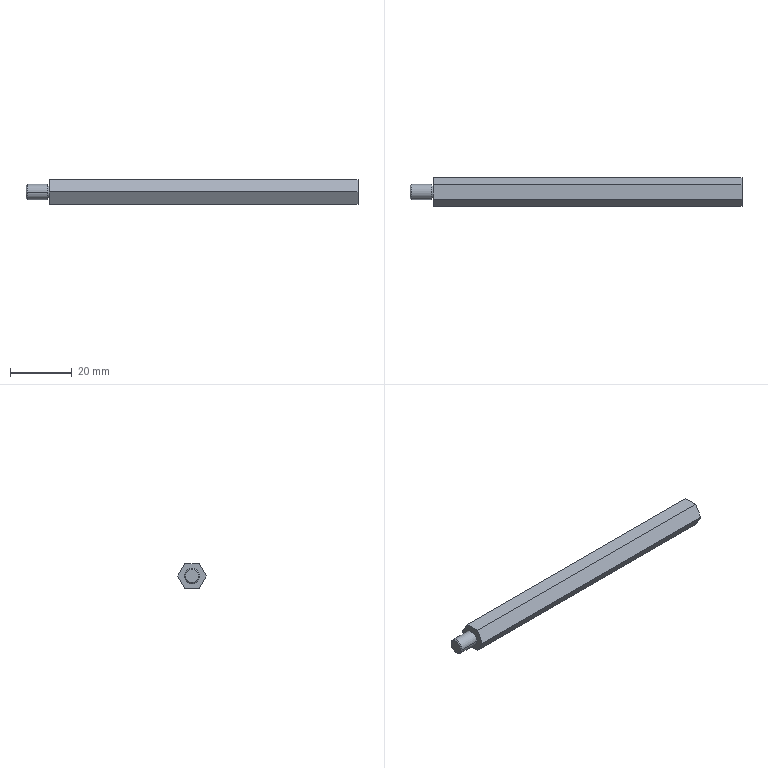Part | NX | 1 solid | 22 faces | box 107.5 x 9.238 x 8 mm | volume 5473 mm3 | plane 10 | cylinder 6 | cone 6 | commonest cylinder face diameters 4.1 x2 4.2 x2 5 x2
STEP:
#1=CARTESIAN_POINT('',(0.,4.619,0.));
#2=VERTEX_POINT('',#1);
#3=CARTESIAN_POINT('',(0.,2.309,4.));
#4=VERTEX_POINT('',#3);
#5=CARTESIAN_POINT('',(0.,4.619,0.));
#6=DIRECTION('',(0.,-0.5,0.866));
#7=VECTOR('',#6,1000.);
#8=LINE('',#5,#7);
#9=EDGE_CURVE('',#2,#4,#8,.T.);
#10=ORIENTED_EDGE('',*,*,#9,.F.);
#11=CARTESIAN_POINT('',(0.,2.309,-4.));
#12=VERTEX_POINT('',#11);
#13=CARTESIAN_POINT('',(0.,2.309,-4.));
#14=DIRECTION('',(0.,0.5,0.866));
#15=VECTOR('',#14,1000.);
#16=LINE('',#13,#15);
#17=EDGE_CURVE('',#12,#2,#16,.T.);
#18=ORIENTED_EDGE('',*,*,#17,.F.);
#19=CARTESIAN_POINT('',(0.,-2.309,-4.));
#20=VERTEX_POINT('',#19);
#21=CARTESIAN_POINT('',(0.,2.309,-4.));
#22=DIRECTION('',(0.,-1.,0.));
#23=VECTOR('',#22,1000.);
#24=LINE('',#21,#23);
#25=EDGE_CURVE('',#12,#20,#24,.T.);
#26=ORIENTED_EDGE('',*,*,#25,.T.);
#27=CARTESIAN_POINT('',(0.,-4.619,0.));
#28=VERTEX_POINT('',#27);
#29=CARTESIAN_POINT('',(0.,-4.619,0.));
#30=DIRECTION('',(0.,0.5,-0.866));
#31=VECTOR('',#30,1000.);
#32=LINE('',#29,#31);
#33=EDGE_CURVE('',#28,#20,#32,.T.);
#34=ORIENTED_EDGE('',*,*,#33,.F.);
#35=CARTESIAN_POINT('',(0.,-2.309,4.));
#36=VERTEX_POINT('',#35);
#37=CARTESIAN_POINT('',(0.,-2.309,4.));
#38=DIRECTION('',(0.,-0.5,-0.866));
#39=VECTOR('',#38,1000.);
#40=LINE('',#37,#39);
#41=EDGE_CURVE('',#36,#28,#40,.T.);
#42=ORIENTED_EDGE('',*,*,#41,.F.);
#43=CARTESIAN_POINT('',(0.,-2.309,4.));
#44=DIRECTION('',(0.,1.,0.));
#45=VECTOR('',#44,1000.);
#46=LINE('',#43,#45);
#47=EDGE_CURVE('',#36,#4,#46,.T.);
#48=ORIENTED_EDGE('',*,*,#47,.T.);
#49=EDGE_LOOP('',(#10,#18,#26,#34,#42,#48));
#50=FACE_BOUND('',#49,.T.);
#51=CARTESIAN_POINT('',(0.,-2.05,0.));
#52=VERTEX_POINT('',#51);
#53=CARTESIAN_POINT('',(0.,2.05,0.));
#54=VERTEX_POINT('',#53);
#55=CARTESIAN_POINT('',(0.,0.,0.));
#56=DIRECTION('',(-1.,0.,0.));
#57=DIRECTION('',(0.,1.,0.));
#58=AXIS2_PLACEMENT_3D('',#55,#56,#57);
#59=CIRCLE('',#58,2.05);
#60=EDGE_CURVE('',#52,#54,#59,.T.);
#61=ORIENTED_EDGE('',*,*,#60,.F.);
#62=CARTESIAN_POINT('',(0.,0.,0.));
#63=DIRECTION('',(-1.,0.,0.));
#64=DIRECTION('',(0.,1.,0.));
#65=AXIS2_PLACEMENT_3D('',#62,#63,#64);
#66=CIRCLE('',#65,2.05);
#67=EDGE_CURVE('',#54,#52,#66,.T.);
#68=ORIENTED_EDGE('',*,*,#67,.F.);
#69=EDGE_LOOP('',(#61,#68));
#70=FACE_BOUND('',#69,.T.);
#71=CARTESIAN_POINT('',(0.,0.,0.));
#72=DIRECTION('',(1.,0.,0.));
#73=DIRECTION('',(0.,1.,0.));
#74=AXIS2_PLACEMENT_3D('',#71,#72,#73);
#75=PLANE('',#74);
#76=ADVANCED_FACE('',(#50,#70),#75,.F.);
#77=ORIENTED_EDGE('',*,*,#9,.T.);
#78=CARTESIAN_POINT('',(100.,2.309,4.));
#79=VERTEX_POINT('',#78);
#80=CARTESIAN_POINT('',(100.,2.309,4.));
#81=DIRECTION('',(-1.,0.,0.));
#82=VECTOR('',#81,1000.);
#83=LINE('',#80,#82);
#84=EDGE_CURVE('',#79,#4,#83,.T.);
#85=ORIENTED_EDGE('',*,*,#84,.F.);
#86=CARTESIAN_POINT('',(100.,4.619,0.));
#87=VERTEX_POINT('',#86);
#88=CARTESIAN_POINT('',(100.,4.619,0.));
#89=DIRECTION('',(0.,0.5,-0.866));
#90=VECTOR('',#89,1000.);
#91=LINE('',#88,#90);
#92=EDGE_CURVE('',#79,#87,#91,.T.);
#93=ORIENTED_EDGE('',*,*,#92,.T.);
#94=CARTESIAN_POINT('',(100.,4.619,0.));
#95=DIRECTION('',(-1.,0.,0.));
#96=VECTOR('',#95,1000.);
#97=LINE('',#94,#96);
#98=EDGE_CURVE('',#87,#2,#97,.T.);
#99=ORIENTED_EDGE('',*,*,#98,.T.);
#100=EDGE_LOOP('',(#77,#85,#93,#99));
#101=FACE_BOUND('',#100,.T.);
#102=CARTESIAN_POINT('',(0.,4.619,0.));
#103=DIRECTION('',(0.,0.866,0.5));
#104=DIRECTION('',(1.,0.,0.));
#105=AXIS2_PLACEMENT_3D('',#102,#103,#104);
#106=PLANE('',#105);
#107=ADVANCED_FACE('',(#101),#106,.T.);
#108=ORIENTED_EDGE('',*,*,#17,.T.);
#109=ORIENTED_EDGE('',*,*,#98,.F.);
#110=CARTESIAN_POINT('',(100.,2.309,-4.));
#111=VERTEX_POINT('',#110);
#112=CARTESIAN_POINT('',(100.,4.619,0.));
#113=DIRECTION('',(0.,-0.5,-0.866));
#114=VECTOR('',#113,1000.);
#115=LINE('',#112,#114);
#116=EDGE_CURVE('',#87,#111,#115,.T.);
#117=ORIENTED_EDGE('',*,*,#116,.T.);
#118=CARTESIAN_POINT('',(100.,2.309,-4.));
#119=DIRECTION('',(-1.,0.,0.));
#120=VECTOR('',#119,1000.);
#121=LINE('',#118,#120);
#122=EDGE_CURVE('',#111,#12,#121,.T.);
#123=ORIENTED_EDGE('',*,*,#122,.T.);
#124=EDGE_LOOP('',(#108,#109,#117,#123));
#125=FACE_BOUND('',#124,.T.);
#126=CARTESIAN_POINT('',(0.,2.309,-4.));
#127=DIRECTION('',(0.,0.866,-0.5));
#128=DIRECTION('',(-1.,0.,0.));
#129=AXIS2_PLACEMENT_3D('',#126,#127,#128);
#130=PLANE('',#129);
#131=ADVANCED_FACE('',(#125),#130,.T.);
#132=ORIENTED_EDGE('',*,*,#25,.F.);
#133=ORIENTED_EDGE('',*,*,#122,.F.);
#134=CARTESIAN_POINT('',(100.,-2.309,-4.));
#135=VERTEX_POINT('',#134);
#136=CARTESIAN_POINT('',(100.,0.,-4.));
#137=DIRECTION('',(0.,-1.,0.));
#138=VECTOR('',#137,1000.);
#139=LINE('',#136,#138);
#140=EDGE_CURVE('',#111,#135,#139,.T.);
#141=ORIENTED_EDGE('',*,*,#140,.T.);
#142=CARTESIAN_POINT('',(100.,-2.309,-4.));
#143=DIRECTION('',(-1.,0.,0.));
#144=VECTOR('',#143,1000.);
#145=LINE('',#142,#144);
#146=EDGE_CURVE('',#135,#20,#145,.T.);
#147=ORIENTED_EDGE('',*,*,#146,.T.);
#148=EDGE_LOOP('',(#132,#133,#141,#147));
#149=FACE_BOUND('',#148,.T.);
#150=CARTESIAN_POINT('',(0.,-2.309,-4.));
#151=DIRECTION('',(0.,0.,-1.));
#152=DIRECTION('',(0.,-1.,0.));
#153=AXIS2_PLACEMENT_3D('',#150,#151,#152);
#154=PLANE('',#153);
#155=ADVANCED_FACE('',(#149),#154,.T.);
#156=ORIENTED_EDGE('',*,*,#33,.T.);
#157=ORIENTED_EDGE('',*,*,#146,.F.);
#158=CARTESIAN_POINT('',(100.,-4.619,0.));
#159=VERTEX_POINT('',#158);
#160=CARTESIAN_POINT('',(100.,-4.619,0.));
#161=DIRECTION('',(0.,-0.5,0.866));
#162=VECTOR('',#161,1000.);
#163=LINE('',#160,#162);
#164=EDGE_CURVE('',#135,#159,#163,.T.);
#165=ORIENTED_EDGE('',*,*,#164,.T.);
#166=CARTESIAN_POINT('',(100.,-4.619,0.));
#167=DIRECTION('',(-1.,0.,0.));
#168=VECTOR('',#167,1000.);
#169=LINE('',#166,#168);
#170=EDGE_CURVE('',#159,#28,#169,.T.);
#171=ORIENTED_EDGE('',*,*,#170,.T.);
#172=EDGE_LOOP('',(#156,#157,#165,#171));
#173=FACE_BOUND('',#172,.T.);
#174=CARTESIAN_POINT('',(0.,-4.619,0.));
#175=DIRECTION('',(0.,-0.866,-0.5));
#176=DIRECTION('',(0.,0.5,-0.866));
#177=AXIS2_PLACEMENT_3D('',#174,#175,#176);
#178=PLANE('',#177);
#179=ADVANCED_FACE('',(#173),#178,.T.);
#180=ORIENTED_EDGE('',*,*,#41,.T.);
#181=ORIENTED_EDGE('',*,*,#170,.F.);
#182=CARTESIAN_POINT('',(100.,-2.309,4.));
#183=VERTEX_POINT('',#182);
#184=CARTESIAN_POINT('',(100.,-4.619,0.));
#185=DIRECTION('',(0.,0.5,0.866));
#186=VECTOR('',#185,1000.);
#187=LINE('',#184,#186);
#188=EDGE_CURVE('',#159,#183,#187,.T.);
#189=ORIENTED_EDGE('',*,*,#188,.T.);
#190=CARTESIAN_POINT('',(100.,-2.309,4.));
#191=DIRECTION('',(-1.,0.,0.));
#192=VECTOR('',#191,1000.);
#193=LINE('',#190,#192);
#194=EDGE_CURVE('',#183,#36,#193,.T.);
#195=ORIENTED_EDGE('',*,*,#194,.T.);
#196=EDGE_LOOP('',(#180,#181,#189,#195));
#197=FACE_BOUND('',#196,.T.);
#198=CARTESIAN_POINT('',(0.,-2.309,4.));
#199=DIRECTION('',(0.,-0.866,0.5));
#200=DIRECTION('',(-1.,0.,0.));
#201=AXIS2_PLACEMENT_3D('',#198,#199,#200);
#202=PLANE('',#201);
#203=ADVANCED_FACE('',(#197),#202,.T.);
#204=ORIENTED_EDGE('',*,*,#47,.F.);
#205=ORIENTED_EDGE('',*,*,#194,.F.);
#206=CARTESIAN_POINT('',(100.,0.,4.));
#207=DIRECTION('',(0.,1.,0.));
#208=VECTOR('',#207,1000.);
#209=LINE('',#206,#208);
#210=EDGE_CURVE('',#183,#79,#209,.T.);
#211=ORIENTED_EDGE('',*,*,#210,.T.);
#212=ORIENTED_EDGE('',*,*,#84,.T.);
#213=EDGE_LOOP('',(#204,#205,#211,#212));
#214=FACE_BOUND('',#213,.T.);
#215=CARTESIAN_POINT('',(0.,2.309,4.));
#216=DIRECTION('',(0.,0.,1.));
#217=DIRECTION('',(1.,0.,0.));
#218=AXIS2_PLACEMENT_3D('',#215,#216,#217);
#219=PLANE('',#218);
#220=ADVANCED_FACE('',(#214),#219,.T.);
#221=ORIENTED_EDGE('',*,*,#92,.F.);
#222=ORIENTED_EDGE('',*,*,#210,.F.);
#223=ORIENTED_EDGE('',*,*,#188,.F.);
#224=ORIENTED_EDGE('',*,*,#164,.F.);
#225=ORIENTED_EDGE('',*,*,#140,.F.);
#226=ORIENTED_EDGE('',*,*,#116,.F.);
#227=EDGE_LOOP('',(#221,#222,#223,#224,#225,#226));
#228=FACE_BOUND('',#227,.T.);
#229=CARTESIAN_POINT('',(100.,-2.86,0.));
#230=VERTEX_POINT('',#229);
#231=CARTESIAN_POINT('',(100.,2.86,0.));
#232=VERTEX_POINT('',#231);
#233=CARTESIAN_POINT('',(100.,0.,0.));
#234=DIRECTION('',(1.,0.,0.));
#235=DIRECTION('',(0.,-1.,0.));
#236=AXIS2_PLACEMENT_3D('',#233,#234,#235);
#237=CIRCLE('',#236,2.86);
#238=EDGE_CURVE('',#230,#232,#237,.T.);
#239=ORIENTED_EDGE('',*,*,#238,.F.);
#240=CARTESIAN_POINT('',(100.,0.,0.));
#241=DIRECTION('',(1.,0.,0.));
#242=DIRECTION('',(0.,-1.,0.));
#243=AXIS2_PLACEMENT_3D('',#240,#241,#242);
#244=CIRCLE('',#243,2.86);
#245=EDGE_CURVE('',#232,#230,#244,.T.);
#246=ORIENTED_EDGE('',*,*,#245,.F.);
#247=EDGE_LOOP('',(#239,#246));
#248=FACE_BOUND('',#247,.T.);
#249=CARTESIAN_POINT('',(100.,0.,0.));
#250=DIRECTION('',(1.,0.,0.));
#251=DIRECTION('',(0.,1.,0.));
#252=AXIS2_PLACEMENT_3D('',#249,#250,#251);
#253=PLANE('',#252);
#254=ADVANCED_FACE('',(#228,#248),#253,.T.);
#255=CARTESIAN_POINT('',(-0.45,-2.5,0.));
#256=VERTEX_POINT('',#255);
#257=CARTESIAN_POINT('',(-0.45,2.5,0.));
#258=VERTEX_POINT('',#257);
#259=CARTESIAN_POINT('',(-0.45,0.,0.));
#260=DIRECTION('',(-1.,0.,0.));
#261=DIRECTION('',(0.,1.,0.));
#262=AXIS2_PLACEMENT_3D('',#259,#260,#261);
#263=CIRCLE('',#262,2.5);
#264=EDGE_CURVE('',#256,#258,#263,.T.);
#265=ORIENTED_EDGE('',*,*,#264,.F.);
#266=CARTESIAN_POINT('',(-0.45,0.,0.));
#267=DIRECTION('',(-1.,0.,0.));
#268=DIRECTION('',(0.,1.,0.));
#269=AXIS2_PLACEMENT_3D('',#266,#267,#268);
#270=CIRCLE('',#269,2.5);
#271=EDGE_CURVE('',#258,#256,#270,.T.);
#272=ORIENTED_EDGE('',*,*,#271,.F.);
#273=EDGE_LOOP('',(#265,#272));
#274=FACE_BOUND('',#273,.T.);
#275=CARTESIAN_POINT('',(-0.45,2.05,0.));
#276=VERTEX_POINT('',#275);
#277=CARTESIAN_POINT('',(-0.45,-2.05,0.));
#278=VERTEX_POINT('',#277);
#279=CARTESIAN_POINT('',(-0.45,0.,0.));
#280=DIRECTION('',(1.,0.,0.));
#281=DIRECTION('',(0.,1.,0.));
#282=AXIS2_PLACEMENT_3D('',#279,#280,#281);
#283=CIRCLE('',#282,2.05);
#284=EDGE_CURVE('',#276,#278,#283,.T.);
#285=ORIENTED_EDGE('',*,*,#284,.F.);
#286=CARTESIAN_POINT('',(-0.45,0.,0.));
#287=DIRECTION('',(1.,0.,0.));
#288=DIRECTION('',(0.,1.,0.));
#289=AXIS2_PLACEMENT_3D('',#286,#287,#288);
#290=CIRCLE('',#289,2.05);
#291=EDGE_CURVE('',#278,#276,#290,.T.);
#292=ORIENTED_EDGE('',*,*,#291,.F.);
#293=EDGE_LOOP('',(#285,#292));
#294=FACE_BOUND('',#293,.T.);
#295=CARTESIAN_POINT('',(-0.45,0.,0.));
#296=DIRECTION('',(1.,0.,0.));
#297=DIRECTION('',(0.,1.,0.));
#298=AXIS2_PLACEMENT_3D('',#295,#296,#297);
#299=PLANE('',#298);
#300=ADVANCED_FACE('',(#274,#294),#299,.T.);
#301=CARTESIAN_POINT('',(-7.5,2.15,0.));
#302=VERTEX_POINT('',#301);
#303=CARTESIAN_POINT('',(-7.5,-2.15,0.));
#304=VERTEX_POINT('',#303);
#305=CARTESIAN_POINT('',(-7.5,0.,0.));
#306=DIRECTION('',(1.,0.,0.));
#307=DIRECTION('',(0.,-1.,0.));
#308=AXIS2_PLACEMENT_3D('',#305,#306,#307);
#309=CIRCLE('',#308,2.15);
#310=EDGE_CURVE('',#302,#304,#309,.T.);
#311=ORIENTED_EDGE('',*,*,#310,.F.);
#312=CARTESIAN_POINT('',(-7.5,0.,0.));
#313=DIRECTION('',(1.,0.,0.));
#314=DIRECTION('',(0.,-1.,0.));
#315=AXIS2_PLACEMENT_3D('',#312,#313,#314);
#316=CIRCLE('',#315,2.15);
#317=EDGE_CURVE('',#304,#302,#316,.T.);
#318=ORIENTED_EDGE('',*,*,#317,.F.);
#319=EDGE_LOOP('',(#311,#318));
#320=FACE_BOUND('',#319,.T.);
#321=CARTESIAN_POINT('',(-7.5,0.,0.));
#322=DIRECTION('',(1.,0.,0.));
#323=DIRECTION('',(0.,1.,0.));
#324=AXIS2_PLACEMENT_3D('',#321,#322,#323);
#325=PLANE('',#324);
#326=ADVANCED_FACE('',(#320),#325,.F.);
#327=ORIENTED_EDGE('',*,*,#264,.T.);
#328=CARTESIAN_POINT('',(-7.15,2.5,0.));
#329=VERTEX_POINT('',#328);
#330=CARTESIAN_POINT('',(-7.875,2.5,0.));
#331=DIRECTION('',(1.,0.,0.));
#332=VECTOR('',#331,1000.);
#333=LINE('',#330,#332);
#334=EDGE_CURVE('',#258,#329,#333,.F.);
#335=ORIENTED_EDGE('',*,*,#334,.T.);
#336=CARTESIAN_POINT('',(-7.15,-2.5,0.));
#337=VERTEX_POINT('',#336);
#338=CARTESIAN_POINT('',(-7.15,0.,0.));
#339=DIRECTION('',(1.,0.,0.));
#340=DIRECTION('',(0.,1.,0.));
#341=AXIS2_PLACEMENT_3D('',#338,#339,#340);
#342=CIRCLE('',#341,2.5);
#343=EDGE_CURVE('',#329,#337,#342,.T.);
#344=ORIENTED_EDGE('',*,*,#343,.T.);
#345=CARTESIAN_POINT('',(-7.875,-2.5,0.));
#346=DIRECTION('',(1.,0.,0.));
#347=VECTOR('',#346,1000.);
#348=LINE('',#345,#347);
#349=EDGE_CURVE('',#256,#337,#348,.F.);
#350=ORIENTED_EDGE('',*,*,#349,.F.);
#351=EDGE_LOOP('',(#327,#335,#344,#350));
#352=FACE_BOUND('',#351,.T.);
#353=CARTESIAN_POINT('',(-7.875,0.,0.));
#354=DIRECTION('',(1.,0.,0.));
#355=DIRECTION('',(0.,-1.,0.));
#356=AXIS2_PLACEMENT_3D('',#353,#354,#355);
#357=CYLINDRICAL_SURFACE('',#356,2.5);
#358=ADVANCED_FACE('',(#352),#357,.T.);
#359=ORIENTED_EDGE('',*,*,#343,.F.);
#360=CARTESIAN_POINT('',(-7.325,2.325,0.));
#361=DIRECTION('',(0.7071,0.7071,0.));
#362=VECTOR('',#361,1000.);
#363=LINE('',#360,#362);
#364=EDGE_CURVE('',#329,#302,#363,.F.);
#365=ORIENTED_EDGE('',*,*,#364,.T.);
#366=ORIENTED_EDGE('',*,*,#310,.T.);
#367=CARTESIAN_POINT('',(-7.325,-2.325,0.));
#368=DIRECTION('',(0.7071,-0.7071,0.));
#369=VECTOR('',#368,1000.);
#370=LINE('',#367,#369);
#371=EDGE_CURVE('',#337,#304,#370,.F.);
#372=ORIENTED_EDGE('',*,*,#371,.F.);
#373=EDGE_LOOP('',(#359,#365,#366,#372));
#374=FACE_BOUND('',#373,.T.);
#375=CARTESIAN_POINT('',(-7.325,0.,0.));
#376=DIRECTION('',(1.,0.,0.));
#377=DIRECTION('',(0.,-1.,0.));
#378=AXIS2_PLACEMENT_3D('',#375,#376,#377);
#379=CONICAL_SURFACE('',#378,2.325,0.7854);
#380=ADVANCED_FACE('',(#374),#379,.T.);
#381=ORIENTED_EDGE('',*,*,#60,.T.);
#382=CARTESIAN_POINT('',(-7.875,2.05,0.));
#383=DIRECTION('',(1.,0.,0.));
#384=VECTOR('',#383,1000.);
#385=LINE('',#382,#384);
#386=EDGE_CURVE('',#54,#276,#385,.F.);
#387=ORIENTED_EDGE('',*,*,#386,.T.);
#388=ORIENTED_EDGE('',*,*,#284,.T.);
#389=CARTESIAN_POINT('',(-7.875,-2.05,0.));
#390=DIRECTION('',(1.,0.,0.));
#391=VECTOR('',#390,1000.);
#392=LINE('',#389,#391);
#393=EDGE_CURVE('',#52,#278,#392,.F.);
#394=ORIENTED_EDGE('',*,*,#393,.F.);
#395=EDGE_LOOP('',(#381,#387,#388,#394));
#396=FACE_BOUND('',#395,.T.);
#397=CARTESIAN_POINT('',(-7.875,0.,0.));
#398=DIRECTION('',(1.,0.,0.));
#399=DIRECTION('',(0.,-1.,0.));
#400=AXIS2_PLACEMENT_3D('',#397,#398,#399);
#401=CYLINDRICAL_SURFACE('',#400,2.05);
#402=ADVANCED_FACE('',(#396),#401,.T.);
#403=CARTESIAN_POINT('',(85.2,2.1,0.));
#404=VERTEX_POINT('',#403);
#405=CARTESIAN_POINT('',(85.2,-2.1,0.));
#406=VERTEX_POINT('',#405);
#407=CARTESIAN_POINT('',(85.2,0.,0.));
#408=DIRECTION('',(1.,0.,0.));
#409=DIRECTION('',(0.,-1.,0.));
#410=AXIS2_PLACEMENT_3D('',#407,#408,#409);
#411=CIRCLE('',#410,2.1);
#412=EDGE_CURVE('',#404,#406,#411,.T.);
#413=ORIENTED_EDGE('',*,*,#412,.F.);
#414=CARTESIAN_POINT('',(99.561,2.1,0.));
#415=VERTEX_POINT('',#414);
#416=CARTESIAN_POINT('',(100.,2.1,0.));
#417=DIRECTION('',(1.,0.,0.));
#418=VECTOR('',#417,1000.);
#419=LINE('',#416,#418);
#420=EDGE_CURVE('',#415,#404,#419,.F.);
#421=ORIENTED_EDGE('',*,*,#420,.F.);
#422=CARTESIAN_POINT('',(99.561,-2.1,0.));
#423=VERTEX_POINT('',#422);
#424=CARTESIAN_POINT('',(99.561,0.,0.));
#425=DIRECTION('',(1.,0.,0.));
#426=DIRECTION('',(0.,-1.,0.));
#427=AXIS2_PLACEMENT_3D('',#424,#425,#426);
#428=CIRCLE('',#427,2.1);
#429=EDGE_CURVE('',#415,#423,#428,.T.);
#430=ORIENTED_EDGE('',*,*,#429,.T.);
#431=CARTESIAN_POINT('',(100.,-2.1,0.));
#432=DIRECTION('',(1.,0.,0.));
#433=VECTOR('',#432,1000.);
#434=LINE('',#431,#433);
#435=EDGE_CURVE('',#423,#406,#434,.F.);
#436=ORIENTED_EDGE('',*,*,#435,.T.);
#437=EDGE_LOOP('',(#413,#421,#430,#436));
#438=FACE_BOUND('',#437,.T.);
#439=CARTESIAN_POINT('',(100.,0.,0.));
#440=DIRECTION('',(1.,0.,0.));
#441=DIRECTION('',(0.,-1.,0.));
#442=AXIS2_PLACEMENT_3D('',#439,#440,#441);
#443=CYLINDRICAL_SURFACE('',#442,2.1);
#444=ADVANCED_FACE('',(#438),#443,.F.);
#445=ORIENTED_EDGE('',*,*,#238,.T.);
#446=CARTESIAN_POINT('',(99.561,2.1,0.));
#447=DIRECTION('',(0.5,0.866,0.));
#448=VECTOR('',#447,1000.);
#449=LINE('',#446,#448);
#450=EDGE_CURVE('',#415,#232,#449,.T.);
#451=ORIENTED_EDGE('',*,*,#450,.F.);
#452=CARTESIAN_POINT('',(99.561,0.,0.));
#453=DIRECTION('',(1.,0.,0.));
#454=DIRECTION('',(0.,-1.,0.));
#455=AXIS2_PLACEMENT_3D('',#452,#453,#454);
#456=CIRCLE('',#455,2.1);
#457=EDGE_CURVE('',#423,#415,#456,.T.);
#458=ORIENTED_EDGE('',*,*,#457,.F.);
#459=CARTESIAN_POINT('',(99.561,-2.1,0.));
#460=DIRECTION('',(0.5,-0.866,0.));
#461=VECTOR('',#460,1000.);
#462=LINE('',#459,#461);
#463=EDGE_CURVE('',#423,#230,#462,.T.);
#464=ORIENTED_EDGE('',*,*,#463,.T.);
#465=EDGE_LOOP('',(#445,#451,#458,#464));
#466=FACE_BOUND('',#465,.T.);
#467=CARTESIAN_POINT('',(99.561,0.,0.));
#468=DIRECTION('',(1.,0.,0.));
#469=DIRECTION('',(0.,-1.,0.));
#470=AXIS2_PLACEMENT_3D('',#467,#468,#469);
#471=CONICAL_SURFACE('',#470,2.1,1.047);
#472=ADVANCED_FACE('',(#466),#471,.F.);
#473=ORIENTED_EDGE('',*,*,#412,.T.);
#474=CARTESIAN_POINT('',(83.938,0.,0.));
#475=VERTEX_POINT('',#474);
#476=CARTESIAN_POINT('',(85.2,-2.1,0.));
#477=DIRECTION('',(0.515,-0.8572,0.));
#478=VECTOR('',#477,1000.);
#479=LINE('',#476,#478);
#480=EDGE_CURVE('',#475,#406,#479,.T.);
#481=ORIENTED_EDGE('',*,*,#480,.F.);
#482=CARTESIAN_POINT('',(85.2,2.1,0.));
#483=DIRECTION('',(0.515,0.8572,0.));
#484=VECTOR('',#483,1000.);
#485=LINE('',#482,#484);
#486=EDGE_CURVE('',#475,#404,#485,.T.);
#487=ORIENTED_EDGE('',*,*,#486,.T.);
#488=EDGE_LOOP('',(#473,#481,#487));
#489=FACE_BOUND('',#488,.T.);
#490=CARTESIAN_POINT('',(85.2,0.,0.));
#491=DIRECTION('',(1.,0.,0.));
#492=DIRECTION('',(0.,-1.,0.));
#493=AXIS2_PLACEMENT_3D('',#490,#491,#492);
#494=CONICAL_SURFACE('',#493,2.1,1.03);
#495=ADVANCED_FACE('',(#489),#494,.F.);
#496=ORIENTED_EDGE('',*,*,#349,.T.);
#497=CARTESIAN_POINT('',(-7.15,0.,0.));
#498=DIRECTION('',(1.,0.,0.));
#499=DIRECTION('',(0.,1.,0.));
#500=AXIS2_PLACEMENT_3D('',#497,#498,#499);
#501=CIRCLE('',#500,2.5);
#502=EDGE_CURVE('',#337,#329,#501,.T.);
#503=ORIENTED_EDGE('',*,*,#502,.T.);
#504=ORIENTED_EDGE('',*,*,#334,.F.);
#505=ORIENTED_EDGE('',*,*,#271,.T.);
#506=EDGE_LOOP('',(#496,#503,#504,#505));
#507=FACE_BOUND('',#506,.T.);
#508=CARTESIAN_POINT('',(-7.875,0.,0.));
#509=DIRECTION('',(1.,0.,0.));
#510=DIRECTION('',(0.,-1.,0.));
#511=AXIS2_PLACEMENT_3D('',#508,#509,#510);
#512=CYLINDRICAL_SURFACE('',#511,2.5);
#513=ADVANCED_FACE('',(#507),#512,.T.);
#514=ORIENTED_EDGE('',*,*,#486,.F.);
#515=ORIENTED_EDGE('',*,*,#480,.T.);
#516=CARTESIAN_POINT('',(85.2,0.,0.));
#517=DIRECTION('',(1.,0.,0.));
#518=DIRECTION('',(0.,-1.,0.));
#519=AXIS2_PLACEMENT_3D('',#516,#517,#518);
#520=CIRCLE('',#519,2.1);
#521=EDGE_CURVE('',#406,#404,#520,.T.);
#522=ORIENTED_EDGE('',*,*,#521,.T.);
#523=EDGE_LOOP('',(#514,#515,#522));
#524=FACE_BOUND('',#523,.T.);
#525=CARTESIAN_POINT('',(85.2,0.,0.));
#526=DIRECTION('',(1.,0.,0.));
#527=DIRECTION('',(0.,-1.,0.));
#528=AXIS2_PLACEMENT_3D('',#525,#526,#527);
#529=CONICAL_SURFACE('',#528,2.1,1.03);
#530=ADVANCED_FACE('',(#524),#529,.F.);
#531=ORIENTED_EDGE('',*,*,#435,.F.);
#532=ORIENTED_EDGE('',*,*,#457,.T.);
#533=ORIENTED_EDGE('',*,*,#420,.T.);
#534=ORIENTED_EDGE('',*,*,#521,.F.);
#535=EDGE_LOOP('',(#531,#532,#533,#534));
#536=FACE_BOUND('',#535,.T.);
#537=CARTESIAN_POINT('',(100.,0.,0.));
#538=DIRECTION('',(1.,0.,0.));
#539=DIRECTION('',(0.,-1.,0.));
#540=AXIS2_PLACEMENT_3D('',#537,#538,#539);
#541=CYLINDRICAL_SURFACE('',#540,2.1);
#542=ADVANCED_FACE('',(#536),#541,.F.);
#543=ORIENTED_EDGE('',*,*,#393,.T.);
#544=ORIENTED_EDGE('',*,*,#291,.T.);
#545=ORIENTED_EDGE('',*,*,#386,.F.);
#546=ORIENTED_EDGE('',*,*,#67,.T.);
#547=EDGE_LOOP('',(#543,#544,#545,#546));
#548=FACE_BOUND('',#547,.T.);
#549=CARTESIAN_POINT('',(-7.875,0.,0.));
#550=DIRECTION('',(1.,0.,0.));
#551=DIRECTION('',(0.,-1.,0.));
#552=AXIS2_PLACEMENT_3D('',#549,#550,#551);
#553=CYLINDRICAL_SURFACE('',#552,2.05);
#554=ADVANCED_FACE('',(#548),#553,.T.);
#555=ORIENTED_EDGE('',*,*,#429,.F.);
#556=ORIENTED_EDGE('',*,*,#450,.T.);
#557=ORIENTED_EDGE('',*,*,#245,.T.);
#558=ORIENTED_EDGE('',*,*,#463,.F.);
#559=EDGE_LOOP('',(#555,#556,#557,#558));
#560=FACE_BOUND('',#559,.T.);
#561=CARTESIAN_POINT('',(99.561,0.,0.));
#562=DIRECTION('',(1.,0.,0.));
#563=DIRECTION('',(0.,-1.,0.));
#564=AXIS2_PLACEMENT_3D('',#561,#562,#563);
#565=CONICAL_SURFACE('',#564,2.1,1.047);
#566=ADVANCED_FACE('',(#560),#565,.F.);
#567=ORIENTED_EDGE('',*,*,#371,.T.);
#568=ORIENTED_EDGE('',*,*,#317,.T.);
#569=ORIENTED_EDGE('',*,*,#364,.F.);
#570=ORIENTED_EDGE('',*,*,#502,.F.);
#571=EDGE_LOOP('',(#567,#568,#569,#570));
#572=FACE_BOUND('',#571,.T.);
#573=CARTESIAN_POINT('',(-7.325,0.,0.));
#574=DIRECTION('',(1.,0.,0.));
#575=DIRECTION('',(0.,-1.,0.));
#576=AXIS2_PLACEMENT_3D('',#573,#574,#575);
#577=CONICAL_SURFACE('',#576,2.325,0.7854);
#578=ADVANCED_FACE('',(#572),#577,.T.);
#579=CLOSED_SHELL('',(#76,#107,#131,#155,#179,#203,#220,#254,#300,#326,#358,#380,#402,#444,#472,#495,#513,#530,#542,#554,#566,#578));
#580=MANIFOLD_SOLID_BREP('',#579);
#581=(LENGTH_UNIT()NAMED_UNIT(*)SI_UNIT(.MILLI.,.METRE.));
#582=UNCERTAINTY_MEASURE_WITH_UNIT(LENGTH_MEASURE(0.00001),#581,'','');
#583=(NAMED_UNIT(*)PLANE_ANGLE_UNIT()SI_UNIT($,.RADIAN.));
#584=(NAMED_UNIT(*)SI_UNIT($,.STERADIAN.)SOLID_ANGLE_UNIT());
#585=(GEOMETRIC_REPRESENTATION_CONTEXT(3)GLOBAL_UNCERTAINTY_ASSIGNED_CONTEXT((#582))GLOBAL_UNIT_ASSIGNED_CONTEXT((#581,#583,#584))REPRESENTATION_CONTEXT('',''));
#586=ADVANCED_BREP_SHAPE_REPRESENTATION('',(#580),#585);